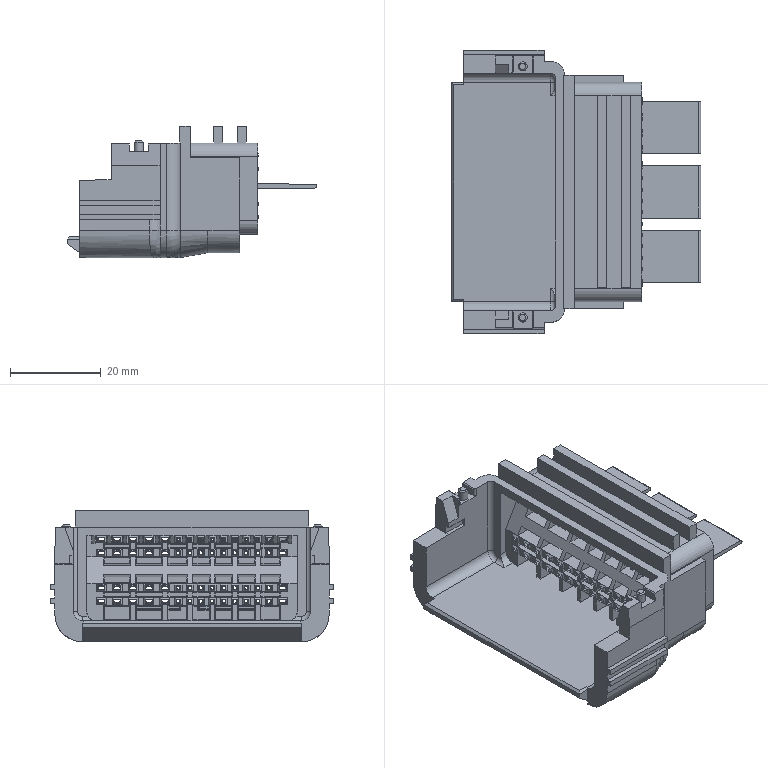Part | NX | features BREP 1 | 1 solid | 7625 faces | volume 25541 mm3 | plane 3719 | cylinder 2811 | torus 614 | sphere 465 | spline 12 | cone 4 | commonest cylinder face diameters 0.09 x1008 1 x481 0.1 x402 0.2 x288 2.01 x288 0.4 x182